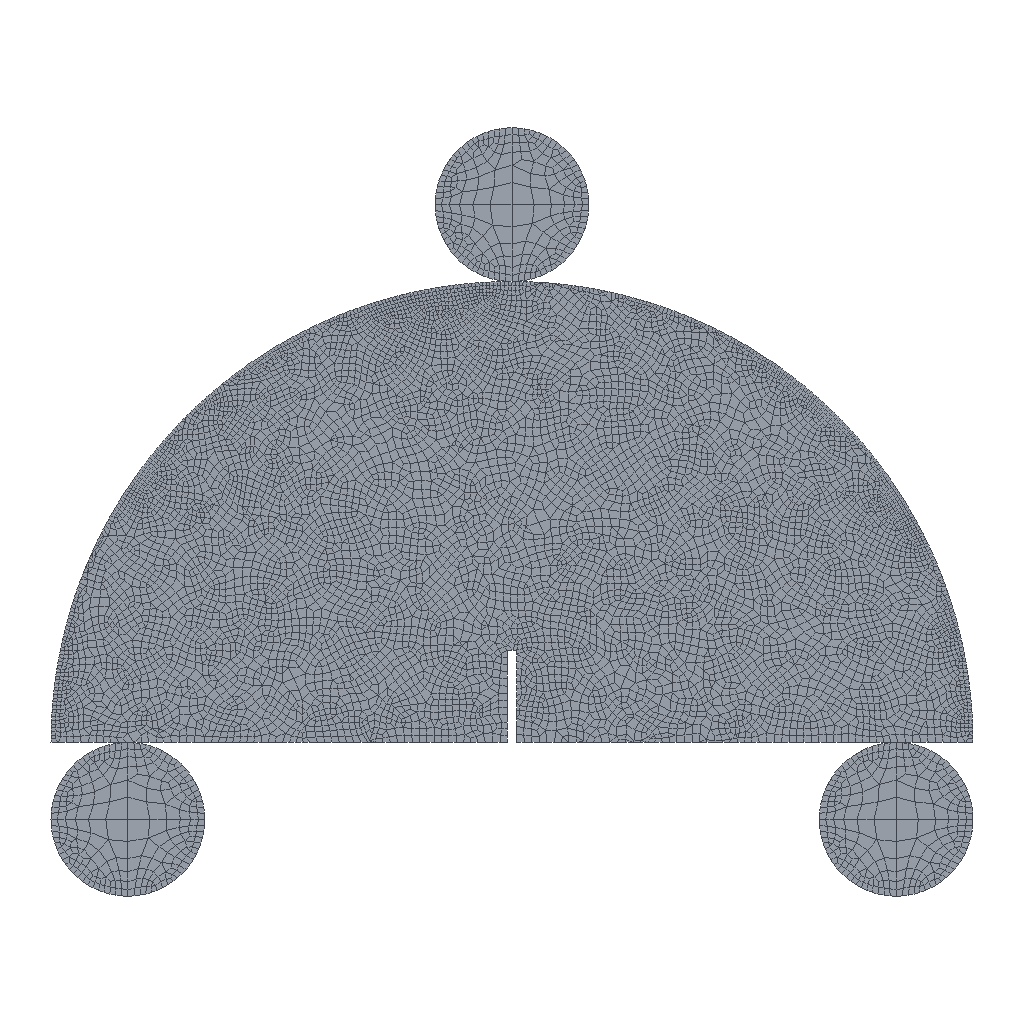Simulation study | abaqus
Set-up summary:
category,name,step,type,value,unit,region
solver,abaqus
solver,version,,,Abaqus/Explicit 2020
units,not stated in the deck,,not stated
analysis,deck,,transient,transient
load_step,Step-1,Step-1,transient,nlgeom=True
contact,interactions,,,general=1 pairs=0 ties=0
load_step,requested,,,1
mesh,nodes,,,28250
mesh,elements,,,21822
element_type,CPS3,,plane,431
element_type,CPS4R,,plane,8869
element_type,COH2D4,,cohesive,12522
load,load commands in deck,,count,1
bc,support commands in deck,,count,6
material,AGG,,in results
material,COH,,in results
material,MAR,,in results
check,setup vs results,,match,"per instance, exact: element labels, types and connectivity; labels of the nodes the elements use; coordinates of those nodes at SINGLE_PRECISION in 4 of 4 instance(s)"
Abaqus input file, long lists of numbers shortened:
*Heading
** Job name: Job-3 Model name: SBS-10
** Generated by: Abaqus/CAE 2020
*Preprint, echo=NO, model=NO, history=NO, contact=NO
**
** PARTS
**
*Part, name=PART-2-SET(JITI)
*Node
    121,         0.75,           0.
    143,          75.,           0.
** (27354 more lines like these left out)
*Element, type=CPS3
  1,  1651,  1635,  1632
  2,  1631,  1651,  1629
** (405 more lines like these left out)
*Element, type=CPS4R
 408,  8591,   680,  1604, 10962
 409,   680,   681,  1605,  1604
** (8111 more lines like these left out)
*Element, type=COH2D4
 8521, 28196, 26040, 26039, 28194
 8522, 25887, 25243, 25241, 25886
** (12520 more lines like these left out)
*Elset, elset=BASEELEMENTS, generate
    1,  8520,     1
*Elset, elset=COHEELEM-0ALL, generate
  8521,  21042,      1
*Elset, elset=COHEELEM-1
  8528,  8544,  8549,  8553,  8565,  8583,  8584,  8601,  8620,  8642,  8655,  8676,  8706,  8709,  8713,  8716
  8726,  8743,  8745,  8754,  8756,  8798,  8802,  8820,  8828,  8834,  8836,  8838,  8840,  8848,  8857,  8869
** (65 more lines like these left out)
*Elset, elset=COHEELEM-2
  8521,  8522,  8523,  8524,  8525,  8526,  8527,  8529,  8530,  8531,  8532,  8533,  8534,  8535,  8536,  8537
  8538,  8539,  8540,  8541,  8542,  8543,  8545,  8546,  8547,  8548,  8550,  8551,  8552,  8554,  8555,  8556
** (714 more lines like these left out)
*Elset, elset=SET-3_COHE
  8521,  8522,  8523,  8524,  8525,  8526,  8527,  8529,  8530,  8531,  8532,  8533,  8534,  8535,  8536,  8537
  8538,  8539,  8540,  8541,  8542,  8543,  8545,  8546,  8547,  8548,  8550,  8551,  8552,  8554,  8555,  8556
** (714 more lines like these left out)
*Elset, elset=JITI_COHE
  8521,  8522,  8523,  8524,  8525,  8526,  8527,  8529,  8530,  8531,  8532,  8533,  8534,  8535,  8536,  8537
  8538,  8539,  8540,  8541,  8542,  8543,  8545,  8546,  8547,  8548,  8550,  8551,  8552,  8554,  8555,  8556
** (714 more lines like these left out)
*Elset, elset=SET-3
   17,   18,   19,   20,   21,   22,   23,   24,   25,   26,   27,   28,   29,   30,   31,   32
   33,   34,   35,   36,   37,   38,   39,   40,   41,   42,   43,   44,   45,   46,   47,   48
** (385 more lines like these left out)
*Elset, elset=GULIAO
    1,    2,    3,    4,    5,    6,    7,    8,    9,   10,   11,   12,   13,   14,   15,   16
  317,  318,  319,  320,  321,  322,  323,  324,  325,  326,  327,  328,  329,  330,  331,  332
** (144 more lines like these left out)
*Elset, elset=JITI
   17,   18,   19,   20,   21,   22,   23,   24,   25,   26,   27,   28,   29,   30,   31,   32
   33,   34,   35,   36,   37,   38,   39,   40,   41,   42,   43,   44,   45,   46,   47,   48
** (385 more lines like these left out)
** Section: Section-1-GULIAO
*Solid Section, elset=GULIAO, material=AGG
11.,
** Section: Section-2-JITI
*Solid Section, elset=JITI, material=MAR
11.,
** Section: Section-3-COHEELEM-0ALL
*Cohesive Section, elset=COHEELEM-0ALL, material=COH, response=TRACTION SEPARATION
, 11.
*End Part
**
*Part, name=PART-5-COPY
*Node
      1,           0.,           0.
      2,         12.5,           0.
** (296 more lines like these left out)
*Element, type=CPS3
1, 117, 123, 113
2, 110, 122, 112
** (6 more lines like these left out)
*Element, type=CPS4R
 3, 111, 125, 119, 108
 4,  16, 106, 115,  15
** (250 more lines like these left out)
*Nset, nset=PART-5-COPY-REFPT_, internal
 298,
*Nset, nset=_PICKEDSET7, internal, generate
   1,  297,    1
*Elset, elset=_PICKEDSET7, internal, generate
   1,  260,    1
** Section: Section-4-_PICKEDSET7
*Solid Section, elset=_PICKEDSET7, material=AGG
11.,
*End Part
**
**
** ASSEMBLY
**
*Assembly, name=Assembly
**
*Instance, name=PART-2-SET(JITI)-1, part=PART-2-SET(JITI)
*End Instance
**
*Instance, name=PART-5-COPY-1, part=PART-5-COPY
       -62.5,        -12.5,           0.
*End Instance
**
*Instance, name=PART-5-COPY-2, part=PART-5-COPY
        62.5,        -12.5,           0.
*End Instance
**
*Instance, name=PART-5-COPY-3, part=PART-5-COPY
          0.,         87.5,           0.
*End Instance
**
*Nset, nset=RP, instance=PART-5-COPY-3
 298,
*Nset, nset=_PICKEDSET45, internal, instance=PART-5-COPY-3
 298,
*Nset, nset=_PICKEDSET46, internal, instance=PART-5-COPY-3, generate
   1,  297,    1
*Elset, elset=_PICKEDSET46, internal, instance=PART-5-COPY-3, generate
   1,  260,    1
*Nset, nset=_PICKEDSET47, internal, instance=PART-5-COPY-1
 298,
*Nset, nset=_PICKEDSET48, internal, instance=PART-5-COPY-1, generate
   1,  297,    1
*Elset, elset=_PICKEDSET48, internal, instance=PART-5-COPY-1, generate
   1,  260,    1
*Nset, nset=_PICKEDSET49, internal, instance=PART-5-COPY-2
 298,
*Nset, nset=_PICKEDSET50, internal, instance=PART-5-COPY-2, generate
   1,  297,    1
*Elset, elset=_PICKEDSET50, internal, instance=PART-5-COPY-2, generate
   1,  260,    1
*Nset, nset=_PICKEDSET52, internal, instance=PART-5-COPY-1
 298,
*Nset, nset=_PICKEDSET52, internal, instance=PART-5-COPY-2
 298,
*Nset, nset=_PickedSet22, internal, instance=PART-5-COPY-3
 298,
*Nset, nset=_PickedSet24, internal, instance=PART-5-COPY-1
 298,
*Nset, nset=_PickedSet26, internal, instance=PART-5-COPY-2
 298,
** Constraint: RigidBody-1
*Rigid Body, ref node=_PickedSet22, elset=_PICKEDSET46
** Constraint: RigidBody-2
*Rigid Body, ref node=_PickedSet24, elset=_PICKEDSET48
** Constraint: RigidBody-3
*Rigid Body, ref node=_PickedSet26, elset=_PICKEDSET50
*End Assembly
*Amplitude, name=AMP-1, definition=SMOOTH STEP
             0.,              0.,           0.005,              1.
**
** MATERIALS
**
*Material, name=AGG
*Density
 2.67e-09,
*Elastic
60000., 0.15
*Material, name=COH
*Damage Initiation, criterion=MAXS
80.,80.,80.
*Damage Evolution, type=ENERGY
 3.349,
*Density
 2e-09,
*Elastic, type=TRACTION
1600.,1600.,1600.
*Material, name=MAR
*Density
 2e-09,
*Elastic, moduli=LONG TERM
 978.194, 0.35
*Viscoelastic, time=PRONY
 0.2874,     0., 0.1713
 0.2606,     0., 0.6489
 0.2363,     0., 6.683
 0.2126,     0., 1254.7
**
** INTERACTION PROPERTIES
**
*Surface Interaction, name=INTPROP-1
*Friction
 0.1,
*Surface Behavior, pressure-overclosure=HARD
**
** BOUNDARY CONDITIONS
**
** Name: Disp-BC-1 Type: 位移/转角
*Boundary
_PICKEDSET52, 1, 1
** Name: Disp-BC-2 Type: 位移/转角
*Boundary
_PICKEDSET52, 2, 2
** Name: Disp-BC-3 Type: 位移/转角
*Boundary
_PICKEDSET52, 6, 6
** ----------------------------------------------------------------
**
** STEP: Step-1
**
*Step, name=Step-1, nlgeom=YES
*Dynamic, Explicit
, 0.005
*Bulk Viscosity
0.06, 1.2
** Mass Scaling: Semi-Automatic
**               Whole Model
*Fixed Mass Scaling, factor=500.
**
** BOUNDARY CONDITIONS
**
** Name: Disp-BC-4 Type: 位移/转角
*Boundary, amplitude=AMP-1
RP, 1, 1
** Name: Disp-BC-5 Type: 位移/转角
*Boundary, amplitude=AMP-1
RP, 2, 2, -3.
** Name: Disp-BC-6 Type: 位移/转角
*Boundary, amplitude=AMP-1
RP, 6, 6
**
** INTERACTIONS
**
** Interaction: general_contact
*Contact, op=NEW
*Contact Inclusions, ALL EXTERIOR
*Contact Property Assignment
 ,  , INTPROP-1
**
** OUTPUT REQUESTS
**
*Restart, write, number interval=1, time marks=NO
**
** FIELD OUTPUT: F-Output-1
**
*Output, field, number interval=50
*Node Output
U,
*Element Output, directions=YES
CFAILURE, DMICRT, LE, S, SDEG, STATUS, SVAVG
*Contact Output
CSTRESS,
**
** HISTORY OUTPUT: H-Output-1
**
*Output, history, variable=PRESELECT
**
** HISTORY OUTPUT: H-Output-2
**
*Output, history, time interval=5e-07
*Node Output, nset=RP
RF2, U2
*End Step
Results summary:
result,step,Step-1,completed,increments=33853 time=0.005/0.005
result,analysis,,,transient
result,last_loadstep,,,1
result,analysis steps,,count,1
result,primary field,,,U